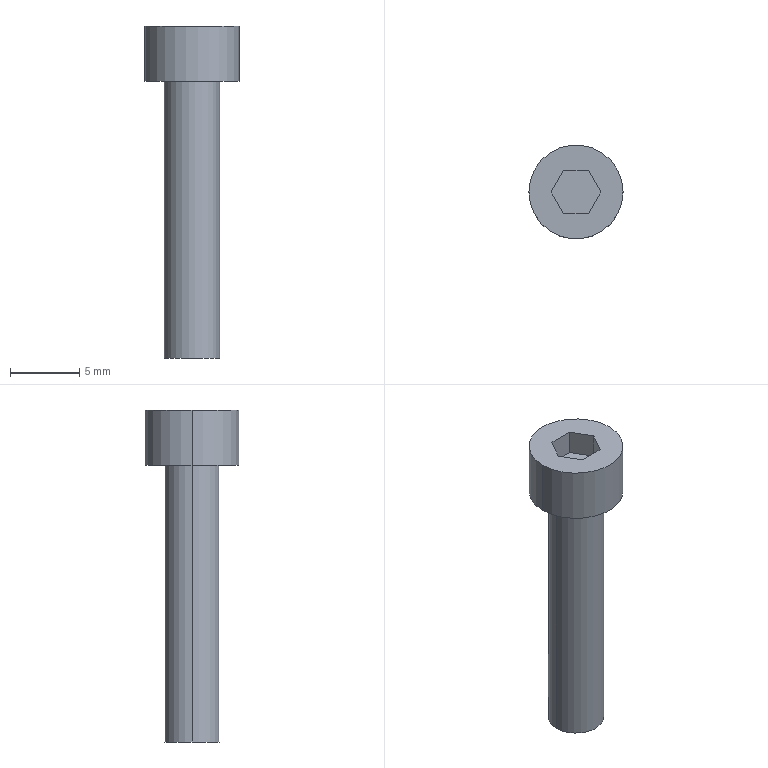Part | SolidWorks | features BaseBody 1 | 1 solid | 14 faces | box 6.8 x 6.8 x 24 mm | volume 381.443 mm3 | plane 10 | cylinder 4 | commonest cylinder face diameters 4 x2 6.8 x2
STEP:
#1=CARTESIAN_POINT('',(2.,0.,-20.));
#2=VERTEX_POINT('',#1);
#3=CARTESIAN_POINT('',(-2.,0.,-20.));
#4=VERTEX_POINT('',#3);
#5=CARTESIAN_POINT('',(0.,0.,-20.));
#6=DIRECTION('',(0.,0.,1.));
#7=DIRECTION('',(1.,0.,0.));
#8=AXIS2_PLACEMENT_3D('',#5,#6,#7);
#9=CIRCLE('',#8,2.);
#10=EDGE_CURVE('',#2,#4,#9,.T.);
#11=ORIENTED_EDGE('',*,*,#10,.T.);
#12=CARTESIAN_POINT('',(-2.,0.,0.));
#13=VERTEX_POINT('',#12);
#14=CARTESIAN_POINT('',(-2.,0.,-20.));
#15=DIRECTION('',(0.,0.,1.));
#16=VECTOR('',#15,1000.);
#17=LINE('',#14,#16);
#18=EDGE_CURVE('',#4,#13,#17,.T.);
#19=ORIENTED_EDGE('',*,*,#18,.T.);
#20=CARTESIAN_POINT('',(2.,0.,0.));
#21=VERTEX_POINT('',#20);
#22=CARTESIAN_POINT('',(0.,0.,0.));
#23=DIRECTION('',(0.,0.,-1.));
#24=DIRECTION('',(1.,0.,0.));
#25=AXIS2_PLACEMENT_3D('',#22,#23,#24);
#26=CIRCLE('',#25,2.);
#27=EDGE_CURVE('',#13,#21,#26,.T.);
#28=ORIENTED_EDGE('',*,*,#27,.T.);
#29=CARTESIAN_POINT('',(2.,0.,-20.));
#30=DIRECTION('',(0.,0.,1.));
#31=VECTOR('',#30,1000.);
#32=LINE('',#29,#31);
#33=EDGE_CURVE('',#2,#21,#32,.T.);
#34=ORIENTED_EDGE('',*,*,#33,.F.);
#35=EDGE_LOOP('',(#11,#19,#28,#34));
#36=FACE_OUTER_BOUND('',#35,.T.);
#37=CARTESIAN_POINT('',(0.,0.,-20.));
#38=DIRECTION('',(0.,0.,1.));
#39=DIRECTION('',(1.,0.,0.));
#40=AXIS2_PLACEMENT_3D('',#37,#38,#39);
#41=CYLINDRICAL_SURFACE('',#40,2.);
#42=ADVANCED_FACE('',(#36),#41,.T.);
#43=CARTESIAN_POINT('',(3.4,0.,0.));
#44=VERTEX_POINT('',#43);
#45=CARTESIAN_POINT('',(-3.4,0.,0.));
#46=VERTEX_POINT('',#45);
#47=CARTESIAN_POINT('',(0.,0.,0.));
#48=DIRECTION('',(0.,0.,1.));
#49=DIRECTION('',(1.,0.,0.));
#50=AXIS2_PLACEMENT_3D('',#47,#48,#49);
#51=CIRCLE('',#50,3.4);
#52=EDGE_CURVE('',#44,#46,#51,.T.);
#53=ORIENTED_EDGE('',*,*,#52,.T.);
#54=CARTESIAN_POINT('',(-3.4,0.,4.));
#55=VERTEX_POINT('',#54);
#56=CARTESIAN_POINT('',(-3.4,0.,0.));
#57=DIRECTION('',(0.,0.,1.));
#58=VECTOR('',#57,1000.);
#59=LINE('',#56,#58);
#60=EDGE_CURVE('',#46,#55,#59,.T.);
#61=ORIENTED_EDGE('',*,*,#60,.T.);
#62=CARTESIAN_POINT('',(3.4,0.,4.));
#63=VERTEX_POINT('',#62);
#64=CARTESIAN_POINT('',(0.,0.,4.));
#65=DIRECTION('',(0.,0.,-1.));
#66=DIRECTION('',(1.,0.,0.));
#67=AXIS2_PLACEMENT_3D('',#64,#65,#66);
#68=CIRCLE('',#67,3.4);
#69=EDGE_CURVE('',#55,#63,#68,.T.);
#70=ORIENTED_EDGE('',*,*,#69,.T.);
#71=CARTESIAN_POINT('',(3.4,0.,0.));
#72=DIRECTION('',(0.,0.,1.));
#73=VECTOR('',#72,1000.);
#74=LINE('',#71,#73);
#75=EDGE_CURVE('',#44,#63,#74,.T.);
#76=ORIENTED_EDGE('',*,*,#75,.F.);
#77=EDGE_LOOP('',(#53,#61,#70,#76));
#78=FACE_OUTER_BOUND('',#77,.T.);
#79=CARTESIAN_POINT('',(0.,0.,0.));
#80=DIRECTION('',(0.,0.,1.));
#81=DIRECTION('',(1.,0.,0.));
#82=AXIS2_PLACEMENT_3D('',#79,#80,#81);
#83=CYLINDRICAL_SURFACE('',#82,3.4);
#84=ADVANCED_FACE('',(#78),#83,.T.);
#85=ORIENTED_EDGE('',*,*,#18,.F.);
#86=CARTESIAN_POINT('',(0.,0.,-20.));
#87=DIRECTION('',(0.,0.,1.));
#88=DIRECTION('',(1.,0.,0.));
#89=AXIS2_PLACEMENT_3D('',#86,#87,#88);
#90=CIRCLE('',#89,2.);
#91=EDGE_CURVE('',#4,#2,#90,.T.);
#92=ORIENTED_EDGE('',*,*,#91,.T.);
#93=ORIENTED_EDGE('',*,*,#33,.T.);
#94=CARTESIAN_POINT('',(0.,0.,0.));
#95=DIRECTION('',(0.,0.,-1.));
#96=DIRECTION('',(1.,0.,0.));
#97=AXIS2_PLACEMENT_3D('',#94,#95,#96);
#98=CIRCLE('',#97,2.);
#99=EDGE_CURVE('',#21,#13,#98,.T.);
#100=ORIENTED_EDGE('',*,*,#99,.T.);
#101=EDGE_LOOP('',(#85,#92,#93,#100));
#102=FACE_OUTER_BOUND('',#101,.T.);
#103=CARTESIAN_POINT('',(0.,0.,-20.));
#104=DIRECTION('',(0.,0.,1.));
#105=DIRECTION('',(1.,0.,0.));
#106=AXIS2_PLACEMENT_3D('',#103,#104,#105);
#107=CYLINDRICAL_SURFACE('',#106,2.);
#108=ADVANCED_FACE('',(#102),#107,.T.);
#109=ORIENTED_EDGE('',*,*,#10,.F.);
#110=ORIENTED_EDGE('',*,*,#91,.F.);
#111=EDGE_LOOP('',(#109,#110));
#112=FACE_OUTER_BOUND('',#111,.T.);
#113=CARTESIAN_POINT('',(0.,0.,-20.));
#114=DIRECTION('',(0.,0.,1.));
#115=DIRECTION('',(1.,0.,0.));
#116=AXIS2_PLACEMENT_3D('',#113,#114,#115);
#117=PLANE('',#116);
#118=ADVANCED_FACE('',(#112),#117,.F.);
#119=ORIENTED_EDGE('',*,*,#99,.F.);
#120=ORIENTED_EDGE('',*,*,#27,.F.);
#121=EDGE_LOOP('',(#119,#120));
#122=FACE_BOUND('',#121,.T.);
#123=ORIENTED_EDGE('',*,*,#52,.F.);
#124=CARTESIAN_POINT('',(0.,0.,0.));
#125=DIRECTION('',(0.,0.,1.));
#126=DIRECTION('',(1.,0.,0.));
#127=AXIS2_PLACEMENT_3D('',#124,#125,#126);
#128=CIRCLE('',#127,3.4);
#129=EDGE_CURVE('',#46,#44,#128,.T.);
#130=ORIENTED_EDGE('',*,*,#129,.F.);
#131=EDGE_LOOP('',(#123,#130));
#132=FACE_OUTER_BOUND('',#131,.T.);
#133=CARTESIAN_POINT('',(0.,0.,0.));
#134=DIRECTION('',(0.,0.,1.));
#135=DIRECTION('',(1.,0.,0.));
#136=AXIS2_PLACEMENT_3D('',#133,#134,#135);
#137=PLANE('',#136);
#138=ADVANCED_FACE('',(#122,#132),#137,.F.);
#139=ORIENTED_EDGE('',*,*,#60,.F.);
#140=ORIENTED_EDGE('',*,*,#129,.T.);
#141=ORIENTED_EDGE('',*,*,#75,.T.);
#142=CARTESIAN_POINT('',(0.,0.,4.));
#143=DIRECTION('',(0.,0.,-1.));
#144=DIRECTION('',(1.,0.,0.));
#145=AXIS2_PLACEMENT_3D('',#142,#143,#144);
#146=CIRCLE('',#145,3.4);
#147=EDGE_CURVE('',#63,#55,#146,.T.);
#148=ORIENTED_EDGE('',*,*,#147,.T.);
#149=EDGE_LOOP('',(#139,#140,#141,#148));
#150=FACE_OUTER_BOUND('',#149,.T.);
#151=CARTESIAN_POINT('',(0.,0.,0.));
#152=DIRECTION('',(0.,0.,1.));
#153=DIRECTION('',(1.,0.,0.));
#154=AXIS2_PLACEMENT_3D('',#151,#152,#153);
#155=CYLINDRICAL_SURFACE('',#154,3.4);
#156=ADVANCED_FACE('',(#150),#155,.T.);
#157=CARTESIAN_POINT('',(-0.9,-1.559,4.));
#158=VERTEX_POINT('',#157);
#159=CARTESIAN_POINT('',(-1.8,0.,4.));
#160=VERTEX_POINT('',#159);
#161=CARTESIAN_POINT('',(-0.9,-1.559,4.));
#162=DIRECTION('',(-0.5,0.866,0.));
#163=VECTOR('',#162,1000.);
#164=LINE('',#161,#163);
#165=EDGE_CURVE('',#158,#160,#164,.T.);
#166=ORIENTED_EDGE('',*,*,#165,.T.);
#167=CARTESIAN_POINT('',(-0.9,1.559,4.));
#168=VERTEX_POINT('',#167);
#169=CARTESIAN_POINT('',(-1.8,0.,4.));
#170=DIRECTION('',(0.5,0.866,0.));
#171=VECTOR('',#170,1000.);
#172=LINE('',#169,#171);
#173=EDGE_CURVE('',#160,#168,#172,.T.);
#174=ORIENTED_EDGE('',*,*,#173,.T.);
#175=CARTESIAN_POINT('',(0.9,1.559,4.));
#176=VERTEX_POINT('',#175);
#177=CARTESIAN_POINT('',(0.,1.559,4.));
#178=DIRECTION('',(1.,0.,0.));
#179=VECTOR('',#178,1000.);
#180=LINE('',#177,#179);
#181=EDGE_CURVE('',#168,#176,#180,.T.);
#182=ORIENTED_EDGE('',*,*,#181,.T.);
#183=CARTESIAN_POINT('',(1.8,0.,4.));
#184=VERTEX_POINT('',#183);
#185=CARTESIAN_POINT('',(0.9,1.559,4.));
#186=DIRECTION('',(0.5,-0.866,0.));
#187=VECTOR('',#186,1000.);
#188=LINE('',#185,#187);
#189=EDGE_CURVE('',#176,#184,#188,.T.);
#190=ORIENTED_EDGE('',*,*,#189,.T.);
#191=CARTESIAN_POINT('',(0.9,-1.559,4.));
#192=VERTEX_POINT('',#191);
#193=CARTESIAN_POINT('',(1.8,0.,4.));
#194=DIRECTION('',(-0.5,-0.866,0.));
#195=VECTOR('',#194,1000.);
#196=LINE('',#193,#195);
#197=EDGE_CURVE('',#184,#192,#196,.T.);
#198=ORIENTED_EDGE('',*,*,#197,.T.);
#199=CARTESIAN_POINT('',(0.,-1.559,4.));
#200=DIRECTION('',(-1.,0.,0.));
#201=VECTOR('',#200,1000.);
#202=LINE('',#199,#201);
#203=EDGE_CURVE('',#192,#158,#202,.T.);
#204=ORIENTED_EDGE('',*,*,#203,.T.);
#205=EDGE_LOOP('',(#166,#174,#182,#190,#198,#204));
#206=FACE_BOUND('',#205,.T.);
#207=ORIENTED_EDGE('',*,*,#147,.F.);
#208=ORIENTED_EDGE('',*,*,#69,.F.);
#209=EDGE_LOOP('',(#207,#208));
#210=FACE_OUTER_BOUND('',#209,.T.);
#211=CARTESIAN_POINT('',(0.,0.,4.));
#212=DIRECTION('',(0.,0.,1.));
#213=DIRECTION('',(1.,0.,0.));
#214=AXIS2_PLACEMENT_3D('',#211,#212,#213);
#215=PLANE('',#214);
#216=ADVANCED_FACE('',(#206,#210),#215,.T.);
#217=ORIENTED_EDGE('',*,*,#173,.F.);
#218=CARTESIAN_POINT('',(-1.8,0.,2.2));
#219=VERTEX_POINT('',#218);
#220=CARTESIAN_POINT('',(-1.8,0.,2.2));
#221=DIRECTION('',(0.,0.,-1.));
#222=VECTOR('',#221,1000.);
#223=LINE('',#220,#222);
#224=EDGE_CURVE('',#160,#219,#223,.T.);
#225=ORIENTED_EDGE('',*,*,#224,.T.);
#226=CARTESIAN_POINT('',(-0.9,1.559,2.2));
#227=VERTEX_POINT('',#226);
#228=CARTESIAN_POINT('',(-0.9,1.559,2.2));
#229=DIRECTION('',(0.5,0.866,0.));
#230=VECTOR('',#229,1000.);
#231=LINE('',#228,#230);
#232=EDGE_CURVE('',#219,#227,#231,.T.);
#233=ORIENTED_EDGE('',*,*,#232,.T.);
#234=CARTESIAN_POINT('',(-0.9,1.559,2.2));
#235=DIRECTION('',(0.,0.,1.));
#236=VECTOR('',#235,1000.);
#237=LINE('',#234,#236);
#238=EDGE_CURVE('',#227,#168,#237,.T.);
#239=ORIENTED_EDGE('',*,*,#238,.T.);
#240=EDGE_LOOP('',(#217,#225,#233,#239));
#241=FACE_OUTER_BOUND('',#240,.T.);
#242=CARTESIAN_POINT('',(-0.9,1.559,2.2));
#243=DIRECTION('',(0.866,-0.5,0.));
#244=DIRECTION('',(0.5,0.866,0.));
#245=AXIS2_PLACEMENT_3D('',#242,#243,#244);
#246=PLANE('',#245);
#247=ADVANCED_FACE('',(#241),#246,.T.);
#248=ORIENTED_EDGE('',*,*,#165,.F.);
#249=CARTESIAN_POINT('',(-0.9,-1.559,2.2));
#250=VERTEX_POINT('',#249);
#251=CARTESIAN_POINT('',(-0.9,-1.559,2.2));
#252=DIRECTION('',(0.,0.,-1.));
#253=VECTOR('',#252,1000.);
#254=LINE('',#251,#253);
#255=EDGE_CURVE('',#158,#250,#254,.T.);
#256=ORIENTED_EDGE('',*,*,#255,.T.);
#257=CARTESIAN_POINT('',(-1.8,0.,2.2));
#258=DIRECTION('',(-0.5,0.866,0.));
#259=VECTOR('',#258,1000.);
#260=LINE('',#257,#259);
#261=EDGE_CURVE('',#250,#219,#260,.T.);
#262=ORIENTED_EDGE('',*,*,#261,.T.);
#263=ORIENTED_EDGE('',*,*,#224,.F.);
#264=EDGE_LOOP('',(#248,#256,#262,#263));
#265=FACE_OUTER_BOUND('',#264,.T.);
#266=CARTESIAN_POINT('',(-1.8,0.,2.2));
#267=DIRECTION('',(0.866,0.5,0.));
#268=DIRECTION('',(-0.5,0.866,0.));
#269=AXIS2_PLACEMENT_3D('',#266,#267,#268);
#270=PLANE('',#269);
#271=ADVANCED_FACE('',(#265),#270,.T.);
#272=ORIENTED_EDGE('',*,*,#203,.F.);
#273=CARTESIAN_POINT('',(0.9,-1.559,2.2));
#274=VERTEX_POINT('',#273);
#275=CARTESIAN_POINT('',(0.9,-1.559,2.2));
#276=DIRECTION('',(0.,0.,-1.));
#277=VECTOR('',#276,1000.);
#278=LINE('',#275,#277);
#279=EDGE_CURVE('',#192,#274,#278,.T.);
#280=ORIENTED_EDGE('',*,*,#279,.T.);
#281=CARTESIAN_POINT('',(-0.9,-1.559,2.2));
#282=DIRECTION('',(-1.,0.,0.));
#283=VECTOR('',#282,1000.);
#284=LINE('',#281,#283);
#285=EDGE_CURVE('',#274,#250,#284,.T.);
#286=ORIENTED_EDGE('',*,*,#285,.T.);
#287=ORIENTED_EDGE('',*,*,#255,.F.);
#288=EDGE_LOOP('',(#272,#280,#286,#287));
#289=FACE_OUTER_BOUND('',#288,.T.);
#290=CARTESIAN_POINT('',(-0.9,-1.559,2.2));
#291=DIRECTION('',(0.,1.,0.));
#292=DIRECTION('',(-1.,0.,0.));
#293=AXIS2_PLACEMENT_3D('',#290,#291,#292);
#294=PLANE('',#293);
#295=ADVANCED_FACE('',(#289),#294,.T.);
#296=ORIENTED_EDGE('',*,*,#197,.F.);
#297=CARTESIAN_POINT('',(1.8,0.,2.2));
#298=VERTEX_POINT('',#297);
#299=CARTESIAN_POINT('',(1.8,0.,2.2));
#300=DIRECTION('',(0.,0.,-1.));
#301=VECTOR('',#300,1000.);
#302=LINE('',#299,#301);
#303=EDGE_CURVE('',#184,#298,#302,.T.);
#304=ORIENTED_EDGE('',*,*,#303,.T.);
#305=CARTESIAN_POINT('',(0.9,-1.559,2.2));
#306=DIRECTION('',(-0.5,-0.866,0.));
#307=VECTOR('',#306,1000.);
#308=LINE('',#305,#307);
#309=EDGE_CURVE('',#298,#274,#308,.T.);
#310=ORIENTED_EDGE('',*,*,#309,.T.);
#311=ORIENTED_EDGE('',*,*,#279,.F.);
#312=EDGE_LOOP('',(#296,#304,#310,#311));
#313=FACE_OUTER_BOUND('',#312,.T.);
#314=CARTESIAN_POINT('',(0.9,-1.559,2.2));
#315=DIRECTION('',(-0.866,0.5,0.));
#316=DIRECTION('',(-0.5,-0.866,0.));
#317=AXIS2_PLACEMENT_3D('',#314,#315,#316);
#318=PLANE('',#317);
#319=ADVANCED_FACE('',(#313),#318,.T.);
#320=ORIENTED_EDGE('',*,*,#189,.F.);
#321=CARTESIAN_POINT('',(0.9,1.559,2.2));
#322=VERTEX_POINT('',#321);
#323=CARTESIAN_POINT('',(0.9,1.559,2.2));
#324=DIRECTION('',(0.,0.,-1.));
#325=VECTOR('',#324,1000.);
#326=LINE('',#323,#325);
#327=EDGE_CURVE('',#176,#322,#326,.T.);
#328=ORIENTED_EDGE('',*,*,#327,.T.);
#329=CARTESIAN_POINT('',(1.8,0.,2.2));
#330=DIRECTION('',(0.5,-0.866,0.));
#331=VECTOR('',#330,1000.);
#332=LINE('',#329,#331);
#333=EDGE_CURVE('',#322,#298,#332,.T.);
#334=ORIENTED_EDGE('',*,*,#333,.T.);
#335=ORIENTED_EDGE('',*,*,#303,.F.);
#336=EDGE_LOOP('',(#320,#328,#334,#335));
#337=FACE_OUTER_BOUND('',#336,.T.);
#338=CARTESIAN_POINT('',(1.8,0.,2.2));
#339=DIRECTION('',(-0.866,-0.5,0.));
#340=DIRECTION('',(0.5,-0.866,0.));
#341=AXIS2_PLACEMENT_3D('',#338,#339,#340);
#342=PLANE('',#341);
#343=ADVANCED_FACE('',(#337),#342,.T.);
#344=ORIENTED_EDGE('',*,*,#181,.F.);
#345=ORIENTED_EDGE('',*,*,#238,.F.);
#346=CARTESIAN_POINT('',(0.9,1.559,2.2));
#347=DIRECTION('',(1.,0.,0.));
#348=VECTOR('',#347,1000.);
#349=LINE('',#346,#348);
#350=EDGE_CURVE('',#227,#322,#349,.T.);
#351=ORIENTED_EDGE('',*,*,#350,.T.);
#352=ORIENTED_EDGE('',*,*,#327,.F.);
#353=EDGE_LOOP('',(#344,#345,#351,#352));
#354=FACE_OUTER_BOUND('',#353,.T.);
#355=CARTESIAN_POINT('',(0.9,1.559,2.2));
#356=DIRECTION('',(0.,-1.,0.));
#357=DIRECTION('',(1.,0.,0.));
#358=AXIS2_PLACEMENT_3D('',#355,#356,#357);
#359=PLANE('',#358);
#360=ADVANCED_FACE('',(#354),#359,.T.);
#361=ORIENTED_EDGE('',*,*,#285,.F.);
#362=ORIENTED_EDGE('',*,*,#309,.F.);
#363=ORIENTED_EDGE('',*,*,#333,.F.);
#364=ORIENTED_EDGE('',*,*,#350,.F.);
#365=ORIENTED_EDGE('',*,*,#232,.F.);
#366=ORIENTED_EDGE('',*,*,#261,.F.);
#367=EDGE_LOOP('',(#361,#362,#363,#364,#365,#366));
#368=FACE_OUTER_BOUND('',#367,.T.);
#369=CARTESIAN_POINT('',(0.,0.,2.2));
#370=DIRECTION('',(0.,0.,1.));
#371=DIRECTION('',(1.,0.,0.));
#372=AXIS2_PLACEMENT_3D('',#369,#370,#371);
#373=PLANE('',#372);
#374=ADVANCED_FACE('',(#368),#373,.T.);
#375=CLOSED_SHELL('',(#42,#84,#108,#118,#138,#156,#216,#247,#271,#295,#319,#343,#360,#374));
#376=MANIFOLD_SOLID_BREP('',#375);
#377=CARTESIAN_POINT('',(0.,0.,0.));
#378=DIRECTION('',(0.,0.,1.));
#379=DIRECTION('',(1.,0.,0.));
#380=AXIS2_PLACEMENT_3D('',#377,#378,#379);
#381=(LENGTH_UNIT()NAMED_UNIT(*)SI_UNIT(.MILLI.,.METRE.));
#382=UNCERTAINTY_MEASURE_WITH_UNIT(LENGTH_MEASURE(0.00001),#381,'','');
#383=(NAMED_UNIT(*)PLANE_ANGLE_UNIT()SI_UNIT($,.RADIAN.));
#384=(NAMED_UNIT(*)SI_UNIT($,.STERADIAN.)SOLID_ANGLE_UNIT());
#385=(GEOMETRIC_REPRESENTATION_CONTEXT(3)GLOBAL_UNCERTAINTY_ASSIGNED_CONTEXT((#382))GLOBAL_UNIT_ASSIGNED_CONTEXT((#381,#383,#384))REPRESENTATION_CONTEXT('',''));
#386=ADVANCED_BREP_SHAPE_REPRESENTATION('',(#376,#380),#385);